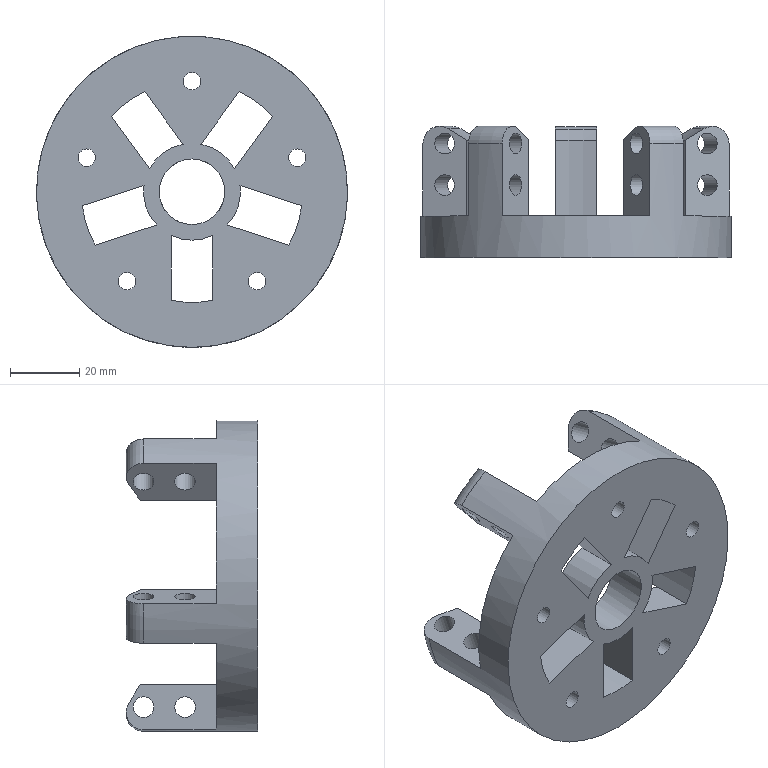Part | NX | features DATUM_CSYS 9, SKETCH 8, EXTRUDE 7, CBORE_HOLE 5, CPROJ 1, HOLE PACKAGE 1, SWP104 1 | 1 solid | 69 faces | box 90 x 38 x 90 mm | volume 71655 mm3 | cylinder 32 | plane 27 | cone 5 | torus 5 | commonest cylinder face diameters 6 x10 5 x5 12 x5 28 x5 64 x5 19 x1